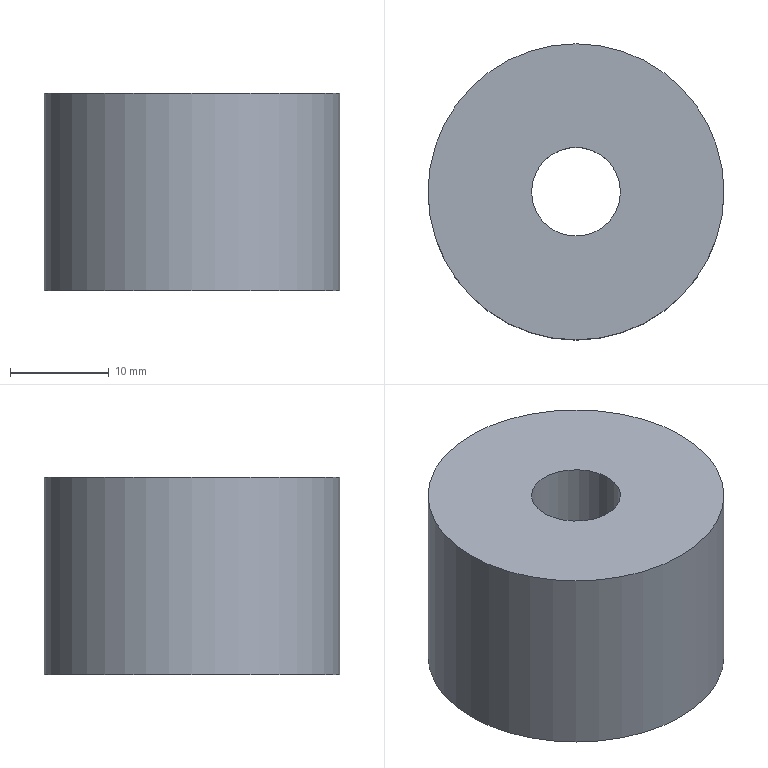Part | STEP file | lll_id2926_x_t | 1 solid | 6 faces | box 30 x 30 x 20 mm | volume 11745 mm3 | plane 3 | cylinder 3 | commonest cylinder face diameters 9.009 x1 14.508 x1 30 x1
STEP:
#1=CARTESIAN_POINT('',(3451.935,184.,20.));
#2=VERTEX_POINT('',#1);
#3=CARTESIAN_POINT('',(3436.935,184.,20.));
#4=DIRECTION('',(0.,0.,1.));
#5=DIRECTION('',(1.,0.,0.));
#6=AXIS2_PLACEMENT_3D('',#3,#4,#5);
#7=CIRCLE('',#6,15.);
#8=EDGE_CURVE('',#2,#2,#7,.T.);
#9=ORIENTED_EDGE('',*,*,#8,.T.);
#10=EDGE_LOOP('',(#9));
#11=FACE_BOUND('',#10,.T.);
#12=CARTESIAN_POINT('',(3441.44,184.,20.));
#13=VERTEX_POINT('',#12);
#14=CARTESIAN_POINT('',(3436.935,184.,20.));
#15=DIRECTION('',(0.,0.,1.));
#16=DIRECTION('',(1.,0.,0.));
#17=AXIS2_PLACEMENT_3D('',#14,#15,#16);
#18=CIRCLE('',#17,4.505);
#19=EDGE_CURVE('',#13,#13,#18,.T.);
#20=ORIENTED_EDGE('',*,*,#19,.F.);
#21=EDGE_LOOP('',(#20));
#22=FACE_BOUND('',#21,.T.);
#23=CARTESIAN_POINT('',(3436.935,184.,20.));
#24=DIRECTION('',(0.,0.,1.));
#25=DIRECTION('',(1.,0.,0.));
#26=AXIS2_PLACEMENT_3D('',#23,#24,#25);
#27=PLANE('',#26);
#28=ADVANCED_FACE('',(#11,#22),#27,.T.);
#29=CARTESIAN_POINT('',(3421.935,184.,0.));
#30=VERTEX_POINT('',#29);
#31=CARTESIAN_POINT('',(3436.935,184.,0.));
#32=DIRECTION('',(0.,0.,-1.));
#33=DIRECTION('',(-1.,0.,0.));
#34=AXIS2_PLACEMENT_3D('',#31,#32,#33);
#35=CIRCLE('',#34,15.);
#36=EDGE_CURVE('',#30,#30,#35,.T.);
#37=ORIENTED_EDGE('',*,*,#36,.T.);
#38=EDGE_LOOP('',(#37));
#39=FACE_BOUND('',#38,.T.);
#40=CARTESIAN_POINT('',(3444.189,184.,0.));
#41=VERTEX_POINT('',#40);
#42=CARTESIAN_POINT('',(3436.935,184.,0.));
#43=DIRECTION('',(0.,0.,-1.));
#44=DIRECTION('',(1.,0.,0.));
#45=AXIS2_PLACEMENT_3D('',#42,#43,#44);
#46=CIRCLE('',#45,7.254);
#47=EDGE_CURVE('',#41,#41,#46,.T.);
#48=ORIENTED_EDGE('',*,*,#47,.F.);
#49=EDGE_LOOP('',(#48));
#50=FACE_BOUND('',#49,.T.);
#51=CARTESIAN_POINT('',(3436.935,184.,0.));
#52=DIRECTION('',(0.,0.,-1.));
#53=DIRECTION('',(-1.,0.,0.));
#54=AXIS2_PLACEMENT_3D('',#51,#52,#53);
#55=PLANE('',#54);
#56=ADVANCED_FACE('',(#39,#50),#55,.T.);
#57=ORIENTED_EDGE('',*,*,#8,.F.);
#58=EDGE_LOOP('',(#57));
#59=FACE_BOUND('',#58,.T.);
#60=ORIENTED_EDGE('',*,*,#36,.F.);
#61=EDGE_LOOP('',(#60));
#62=FACE_BOUND('',#61,.T.);
#63=CARTESIAN_POINT('',(3436.935,184.,0.));
#64=DIRECTION('',(0.,0.,1.));
#65=DIRECTION('',(1.,0.,0.));
#66=AXIS2_PLACEMENT_3D('',#63,#64,#65);
#67=CYLINDRICAL_SURFACE('',#66,15.);
#68=ADVANCED_FACE('',(#59,#62),#67,.T.);
#69=CARTESIAN_POINT('',(3441.44,184.,11.));
#70=VERTEX_POINT('',#69);
#71=CARTESIAN_POINT('',(3436.935,184.,11.));
#72=DIRECTION('',(0.,0.,-1.));
#73=DIRECTION('',(1.,0.,0.));
#74=AXIS2_PLACEMENT_3D('',#71,#72,#73);
#75=CIRCLE('',#74,4.505);
#76=EDGE_CURVE('',#70,#70,#75,.T.);
#77=ORIENTED_EDGE('',*,*,#76,.T.);
#78=EDGE_LOOP('',(#77));
#79=FACE_BOUND('',#78,.T.);
#80=ORIENTED_EDGE('',*,*,#19,.T.);
#81=EDGE_LOOP('',(#80));
#82=FACE_BOUND('',#81,.T.);
#83=CARTESIAN_POINT('',(3436.935,184.,0.));
#84=DIRECTION('',(0.,0.,1.));
#85=DIRECTION('',(1.,0.,0.));
#86=AXIS2_PLACEMENT_3D('',#83,#84,#85);
#87=CYLINDRICAL_SURFACE('',#86,4.505);
#88=ADVANCED_FACE('',(#79,#82),#87,.F.);
#89=ORIENTED_EDGE('',*,*,#76,.F.);
#90=EDGE_LOOP('',(#89));
#91=FACE_BOUND('',#90,.T.);
#92=CARTESIAN_POINT('',(3444.189,184.,11.));
#93=VERTEX_POINT('',#92);
#94=CARTESIAN_POINT('',(3436.935,184.,11.));
#95=DIRECTION('',(0.,0.,-1.));
#96=DIRECTION('',(1.,0.,0.));
#97=AXIS2_PLACEMENT_3D('',#94,#95,#96);
#98=CIRCLE('',#97,7.254);
#99=EDGE_CURVE('',#93,#93,#98,.T.);
#100=ORIENTED_EDGE('',*,*,#99,.T.);
#101=EDGE_LOOP('',(#100));
#102=FACE_BOUND('',#101,.T.);
#103=CARTESIAN_POINT('',(3436.935,184.,11.));
#104=DIRECTION('',(0.,0.,1.));
#105=DIRECTION('',(1.,0.,0.));
#106=AXIS2_PLACEMENT_3D('',#103,#104,#105);
#107=PLANE('',#106);
#108=ADVANCED_FACE('',(#91,#102),#107,.F.);
#109=ORIENTED_EDGE('',*,*,#99,.F.);
#110=EDGE_LOOP('',(#109));
#111=FACE_BOUND('',#110,.T.);
#112=ORIENTED_EDGE('',*,*,#47,.T.);
#113=EDGE_LOOP('',(#112));
#114=FACE_BOUND('',#113,.T.);
#115=CARTESIAN_POINT('',(3436.935,184.,0.));
#116=DIRECTION('',(0.,0.,1.));
#117=DIRECTION('',(1.,0.,0.));
#118=AXIS2_PLACEMENT_3D('',#115,#116,#117);
#119=CYLINDRICAL_SURFACE('',#118,7.254);
#120=ADVANCED_FACE('',(#111,#114),#119,.F.);
#121=CLOSED_SHELL('',(#28,#56,#68,#88,#108,#120));
#122=MANIFOLD_SOLID_BREP('',#121);
#123=(LENGTH_UNIT()NAMED_UNIT(*)SI_UNIT(.MILLI.,.METRE.));
#124=UNCERTAINTY_MEASURE_WITH_UNIT(LENGTH_MEASURE(0.00002),#123,'','');
#125=(NAMED_UNIT(*)PLANE_ANGLE_UNIT()SI_UNIT($,.RADIAN.));
#126=PLANE_ANGLE_MEASURE_WITH_UNIT(PLANE_ANGLE_MEASURE(0.01745),#125);
#127=DIMENSIONAL_EXPONENTS(0.,0.,0.,0.,0.,0.,0.);
#128=(CONVERSION_BASED_UNIT('DEGREE',#126)NAMED_UNIT(#127)PLANE_ANGLE_UNIT());
#129=(NAMED_UNIT(*)SI_UNIT($,.STERADIAN.)SOLID_ANGLE_UNIT());
#130=(GEOMETRIC_REPRESENTATION_CONTEXT(3)GLOBAL_UNCERTAINTY_ASSIGNED_CONTEXT((#124))GLOBAL_UNIT_ASSIGNED_CONTEXT((#123,#128,#129))REPRESENTATION_CONTEXT('',''));
#131=ADVANCED_BREP_SHAPE_REPRESENTATION('',(#122),#130);